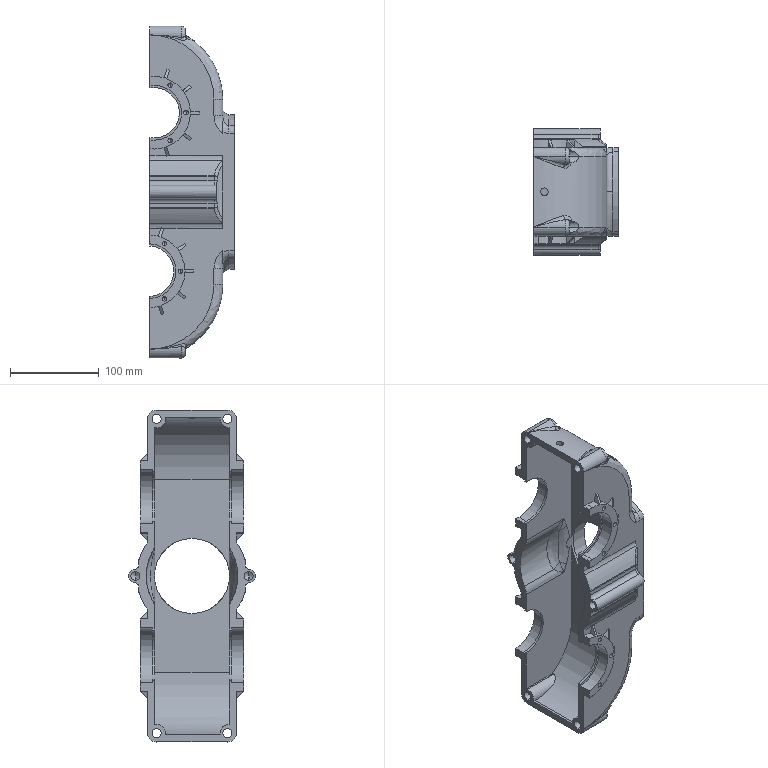Part | SolidWorks | features BaseBody 1, ICE 1 | 1 solid | 379 faces | box 95.5 x 143.009 x 375 mm | volume 902272 mm3 | cylinder 160 | plane 110 | spline 54 | cone 48 | sphere 4 | torus 3 | commonest cylinder face diameters 82 x26 5 x24 20 x23 6.8 x12 10 x12 10.2 x12